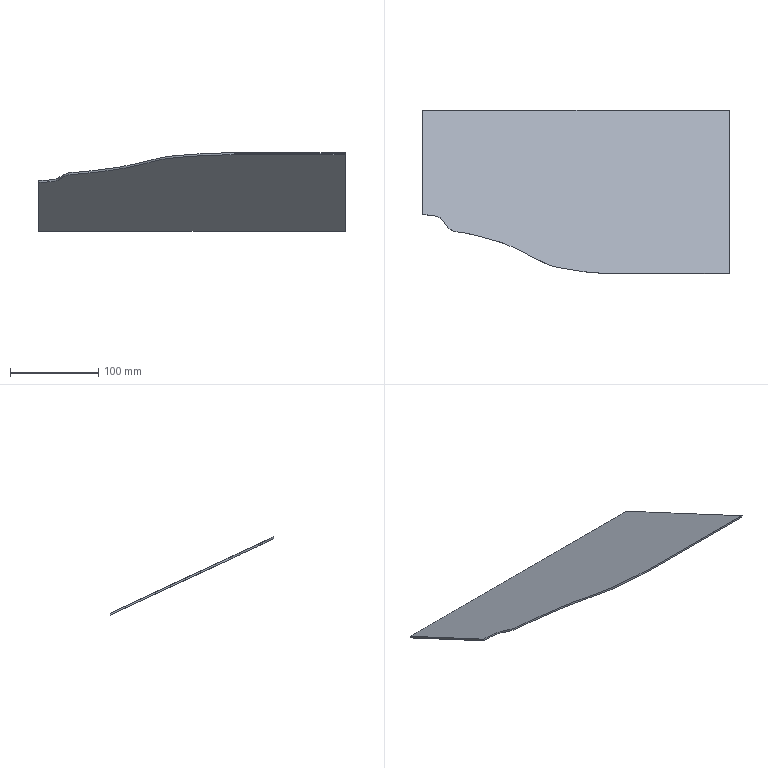Part | NX | features solid 2 | 1 solid | 7 faces | box 347.317 x 185.12 x 88.474 mm | volume 129371 mm3 | plane 6 | spline 1
STEP:
#1=CARTESIAN_POINT('',(-687.317,420.,-186.267));
#2=VERTEX_POINT('',#1);
#3=CARTESIAN_POINT('',(-687.317,420.,-188.474));
#4=VERTEX_POINT('',#3);
#5=CARTESIAN_POINT('',(-687.317,420.,-278.543));
#6=DIRECTION('',(0.,0.,-1.));
#7=VECTOR('',#6,1000.);
#8=LINE('',#5,#7);
#9=EDGE_CURVE('',#2,#4,#8,.T.);
#10=ORIENTED_EDGE('',*,*,#9,.F.);
#11=CARTESIAN_POINT('',(-340.,420.,-186.267));
#12=VERTEX_POINT('',#11);
#13=CARTESIAN_POINT('',(-330.,420.,-186.267));
#14=DIRECTION('',(-1.,0.,0.));
#15=VECTOR('',#14,1000.);
#16=LINE('',#13,#15);
#17=EDGE_CURVE('',#12,#2,#16,.T.);
#18=ORIENTED_EDGE('',*,*,#17,.F.);
#19=CARTESIAN_POINT('',(-340.,420.,-188.474));
#20=VERTEX_POINT('',#19);
#21=CARTESIAN_POINT('',(-340.,420.,10.));
#22=DIRECTION('',(0.,0.,-1.));
#23=VECTOR('',#22,1000.);
#24=LINE('',#21,#23);
#25=EDGE_CURVE('',#12,#20,#24,.T.);
#26=ORIENTED_EDGE('',*,*,#25,.T.);
#27=CARTESIAN_POINT('',(-330.,420.,-188.474));
#28=DIRECTION('',(-1.,0.,0.));
#29=VECTOR('',#28,1000.);
#30=LINE('',#27,#29);
#31=EDGE_CURVE('',#20,#4,#30,.T.);
#32=ORIENTED_EDGE('',*,*,#31,.T.);
#33=EDGE_LOOP('',(#10,#18,#26,#32));
#34=FACE_BOUND('',#33,.T.);
#35=CARTESIAN_POINT('',(0.,420.,10.));
#36=DIRECTION('',(0.,1.,0.));
#37=DIRECTION('',(0.,0.,1.));
#38=AXIS2_PLACEMENT_3D('',#35,#36,#37);
#39=PLANE('',#38);
#40=ADVANCED_FACE('',(#34),#39,.T.);
#41=CARTESIAN_POINT('',(-340.,234.931,-102.175));
#42=VERTEX_POINT('',#41);
#43=CARTESIAN_POINT('',(-340.,234.931,-100.147));
#44=VERTEX_POINT('',#43);
#45=CARTESIAN_POINT('',(-340.,234.931,610.));
#46=DIRECTION('',(0.,0.,-1.));
#47=VECTOR('',#46,1000.);
#48=LINE('',#45,#47);
#49=EDGE_CURVE('',#42,#44,#48,.F.);
#50=ORIENTED_EDGE('',*,*,#49,.F.);
#51=CARTESIAN_POINT('',(-340.,259.69,-113.72));
#52=DIRECTION('',(0.,-0.9063,0.4226));
#53=VECTOR('',#52,1000.);
#54=LINE('',#51,#53);
#55=EDGE_CURVE('',#20,#42,#54,.T.);
#56=ORIENTED_EDGE('',*,*,#55,.F.);
#57=ORIENTED_EDGE('',*,*,#25,.F.);
#58=CARTESIAN_POINT('',(-340.,235.,-100.));
#59=VERTEX_POINT('',#58);
#60=CARTESIAN_POINT('',(-340.,260.535,-111.907));
#61=DIRECTION('',(0.,-0.9063,0.4226));
#62=VECTOR('',#61,1000.);
#63=LINE('',#60,#62);
#64=EDGE_CURVE('',#12,#59,#63,.T.);
#65=ORIENTED_EDGE('',*,*,#64,.T.);
#66=CARTESIAN_POINT('',(-340.,204.395,-165.633));
#67=DIRECTION('',(0.,0.4226,0.9063));
#68=VECTOR('',#67,1000.);
#69=LINE('',#66,#68);
#70=EDGE_CURVE('',#59,#44,#69,.F.);
#71=ORIENTED_EDGE('',*,*,#70,.T.);
#72=EDGE_LOOP('',(#50,#56,#57,#65,#71));
#73=FACE_BOUND('',#72,.T.);
#74=CARTESIAN_POINT('',(-340.,229.93,-177.54));
#75=DIRECTION('',(1.,0.,0.));
#76=DIRECTION('',(0.,1.,0.));
#77=AXIS2_PLACEMENT_3D('',#74,#75,#76);
#78=PLANE('',#77);
#79=ADVANCED_FACE('',(#73),#78,.T.);
#80=CARTESIAN_POINT('',(-480.341,235.,-100.));
#81=VERTEX_POINT('',#80);
#82=CARTESIAN_POINT('',(-340.,234.931,-100.147));
#83=CARTESIAN_POINT('',(-351.695,234.929,-100.153));
#84=CARTESIAN_POINT('',(-369.238,234.931,-100.149));
#85=CARTESIAN_POINT('',(-392.628,234.933,-100.144));
#86=CARTESIAN_POINT('',(-410.171,234.936,-100.138));
#87=CARTESIAN_POINT('',(-427.714,234.923,-100.164));
#88=CARTESIAN_POINT('',(-445.256,234.981,-100.04));
#89=CARTESIAN_POINT('',(-462.799,234.921,-100.169));
#90=CARTESIAN_POINT('',(-474.494,234.863,-100.294));
#91=CARTESIAN_POINT('',(-480.341,235.,-100.));
#92=B_SPLINE_CURVE_WITH_KNOTS('',3,(#82,#83,#84,#85,#86,#87,#88,#89,#90,#91),.UNSPECIFIED.,.F.,.F.,(4,1,1,1,1,1,1,4),(0.,0.03509,0.05263,0.07017,0.08771,0.1053,0.1228,0.1403),.UNSPECIFIED.);
#93=EDGE_CURVE('',#44,#81,#92,.T.);
#94=ORIENTED_EDGE('',*,*,#93,.F.);
#95=ORIENTED_EDGE('',*,*,#70,.F.);
#96=CARTESIAN_POINT('',(-330.,235.,-100.));
#97=DIRECTION('',(-1.,0.,0.));
#98=VECTOR('',#97,1000.);
#99=LINE('',#96,#98);
#100=EDGE_CURVE('',#59,#81,#99,.T.);
#101=ORIENTED_EDGE('',*,*,#100,.T.);
#102=EDGE_LOOP('',(#94,#95,#101));
#103=FACE_BOUND('',#102,.T.);
#104=CARTESIAN_POINT('',(-330.,235.,-100.));
#105=DIRECTION('',(0.,0.9063,-0.4226));
#106=DIRECTION('',(-1.,0.,0.));
#107=AXIS2_PLACEMENT_3D('',#104,#105,#106);
#108=PLANE('',#107);
#109=ADVANCED_FACE('',(#103),#108,.F.);
#110=ORIENTED_EDGE('',*,*,#55,.T.);
#111=CARTESIAN_POINT('',(-687.317,301.902,-133.404));
#112=VERTEX_POINT('',#111);
#113=CARTESIAN_POINT('',(-340.,234.931,-102.175));
#114=CARTESIAN_POINT('',(-355.074,234.928,-102.173));
#115=CARTESIAN_POINT('',(-377.686,234.93,-102.174));
#116=CARTESIAN_POINT('',(-407.834,234.937,-102.178));
#117=CARTESIAN_POINT('',(-430.446,234.919,-102.169));
#118=CARTESIAN_POINT('',(-453.054,235.016,-102.214));
#119=CARTESIAN_POINT('',(-475.676,234.729,-102.08));
#120=CARTESIAN_POINT('',(-494.491,235.465,-102.424));
#121=CARTESIAN_POINT('',(-509.495,237.573,-103.406));
#122=CARTESIAN_POINT('',(-520.718,239.567,-104.336));
#123=CARTESIAN_POINT('',(-532.008,241.304,-105.147));
#124=CARTESIAN_POINT('',(-543.033,243.631,-106.231));
#125=CARTESIAN_POINT('',(-552.986,248.236,-108.379));
#126=CARTESIAN_POINT('',(-562.547,253.682,-110.918));
#127=CARTESIAN_POINT('',(-572.273,258.772,-113.292));
#128=CARTESIAN_POINT('',(-582.129,263.597,-115.542));
#129=CARTESIAN_POINT('',(-592.142,268.098,-117.64));
#130=CARTESIAN_POINT('',(-602.583,271.723,-119.331));
#131=CARTESIAN_POINT('',(-613.442,274.478,-120.616));
#132=CARTESIAN_POINT('',(-622.441,276.919,-121.754));
#133=CARTESIAN_POINT('',(-629.618,278.958,-122.705));
#134=CARTESIAN_POINT('',(-635.058,280.282,-123.322));
#135=CARTESIAN_POINT('',(-640.652,281.056,-123.683));
#136=CARTESIAN_POINT('',(-646.334,281.543,-123.91));
#137=CARTESIAN_POINT('',(-651.889,282.377,-124.299));
#138=CARTESIAN_POINT('',(-657.063,284.955,-125.501));
#139=CARTESIAN_POINT('',(-660.894,289.817,-127.768));
#140=CARTESIAN_POINT('',(-664.331,295.331,-130.34));
#141=CARTESIAN_POINT('',(-668.804,299.109,-132.101));
#142=CARTESIAN_POINT('',(-674.604,300.662,-132.826));
#143=CARTESIAN_POINT('',(-681.069,301.1,-133.03));
#144=CARTESIAN_POINT('',(-685.257,301.597,-133.261));
#145=CARTESIAN_POINT('',(-687.317,301.902,-133.404));
#146=B_SPLINE_CURVE_WITH_KNOTS('',3,(#113,#114,#115,#116,#117,#118,#119,#120,#121,#122,#123,#124,#125,#126,#127,#128,#129,#130,#131,#132,#133,#134,#135,#136,#137,#138,#139,#140,#141,#142,#143,#144,#145),.UNSPECIFIED.,.F.,.F.,(4,1,1,1,1,1,1,1,1,1,1,1,1,1,1,1,1,1,1,1,1,1,1,1,1,1,1,1,1,1,4),(0.,0.0452,0.0678,0.0904,0.113,0.1356,0.1582,0.1695,0.1808,0.1921,0.2034,0.2147,0.226,0.2373,0.2486,0.2599,0.2712,0.2825,0.2938,0.2994,0.3051,0.3107,0.3164,0.322,0.3277,0.3333,0.339,0.3446,0.3503,0.3559,0.3616),.UNSPECIFIED.);
#147=EDGE_CURVE('',#42,#112,#146,.T.);
#148=ORIENTED_EDGE('',*,*,#147,.T.);
#149=CARTESIAN_POINT('',(-687.317,596.678,-270.86));
#150=DIRECTION('',(0.,-0.9063,0.4226));
#151=VECTOR('',#150,1000.);
#152=LINE('',#149,#151);
#153=EDGE_CURVE('',#4,#112,#152,.T.);
#154=ORIENTED_EDGE('',*,*,#153,.F.);
#155=ORIENTED_EDGE('',*,*,#31,.F.);
#156=EDGE_LOOP('',(#110,#148,#154,#155));
#157=FACE_BOUND('',#156,.T.);
#158=CARTESIAN_POINT('',(-330.,596.678,-270.86));
#159=DIRECTION('',(0.,0.4226,0.9063));
#160=DIRECTION('',(1.,0.,0.));
#161=AXIS2_PLACEMENT_3D('',#158,#159,#160);
#162=PLANE('',#161);
#163=ADVANCED_FACE('',(#157),#162,.F.);
#164=CARTESIAN_POINT('',(-687.317,301.902,-131.197));
#165=VERTEX_POINT('',#164);
#166=CARTESIAN_POINT('',(-687.317,301.902,-133.808));
#167=DIRECTION('',(0.,0.,-1.));
#168=VECTOR('',#167,1000.);
#169=LINE('',#166,#168);
#170=EDGE_CURVE('',#165,#112,#169,.T.);
#171=ORIENTED_EDGE('',*,*,#170,.F.);
#172=CARTESIAN_POINT('',(-687.317,597.523,-269.047));
#173=DIRECTION('',(0.,-0.9063,0.4226));
#174=VECTOR('',#173,1000.);
#175=LINE('',#172,#174);
#176=EDGE_CURVE('',#2,#165,#175,.T.);
#177=ORIENTED_EDGE('',*,*,#176,.F.);
#178=ORIENTED_EDGE('',*,*,#9,.T.);
#179=ORIENTED_EDGE('',*,*,#153,.T.);
#180=EDGE_LOOP('',(#171,#177,#178,#179));
#181=FACE_BOUND('',#180,.T.);
#182=CARTESIAN_POINT('',(-687.317,415.853,-278.543));
#183=DIRECTION('',(-1.,0.,0.));
#184=DIRECTION('',(0.,0.,1.));
#185=AXIS2_PLACEMENT_3D('',#182,#183,#184);
#186=PLANE('',#185);
#187=ADVANCED_FACE('',(#181),#186,.T.);
#188=CARTESIAN_POINT('',(-480.341,235.,-100.));
#189=CARTESIAN_POINT('',(-485.184,235.114,-100.053));
#190=CARTESIAN_POINT('',(-494.831,235.59,-100.275));
#191=CARTESIAN_POINT('',(-509.128,237.47,-101.152));
#192=CARTESIAN_POINT('',(-520.955,239.594,-102.142));
#193=CARTESIAN_POINT('',(-530.45,241.116,-102.852));
#194=CARTESIAN_POINT('',(-537.531,242.404,-103.453));
#195=CARTESIAN_POINT('',(-544.264,244.33,-104.351));
#196=CARTESIAN_POINT('',(-550.56,247.084,-105.635));
#197=CARTESIAN_POINT('',(-556.599,250.322,-107.145));
#198=CARTESIAN_POINT('',(-564.584,254.766,-109.217));
#199=CARTESIAN_POINT('',(-574.719,260.029,-111.671));
#200=CARTESIAN_POINT('',(-587.087,265.966,-114.44));
#201=CARTESIAN_POINT('',(-599.843,271.007,-116.79));
#202=CARTESIAN_POINT('',(-611.053,273.879,-118.13));
#203=CARTESIAN_POINT('',(-620.004,276.226,-119.224));
#204=CARTESIAN_POINT('',(-626.681,278.134,-120.114));
#205=CARTESIAN_POINT('',(-633.375,279.968,-120.969));
#206=CARTESIAN_POINT('',(-640.261,281.063,-121.48));
#207=CARTESIAN_POINT('',(-647.289,281.562,-121.712));
#208=CARTESIAN_POINT('',(-652.977,282.75,-122.266));
#209=CARTESIAN_POINT('',(-656.843,285.163,-123.391));
#210=CARTESIAN_POINT('',(-659.875,288.303,-124.856));
#211=CARTESIAN_POINT('',(-662.704,292.92,-127.009));
#212=CARTESIAN_POINT('',(-666.161,297.202,-129.005));
#213=CARTESIAN_POINT('',(-670.181,299.408,-130.034));
#214=CARTESIAN_POINT('',(-674.613,300.635,-130.606));
#215=CARTESIAN_POINT('',(-680.434,301.053,-130.801));
#216=CARTESIAN_POINT('',(-685.03,301.563,-131.039));
#217=CARTESIAN_POINT('',(-687.317,301.902,-131.197));
#218=B_SPLINE_CURVE_WITH_KNOTS('',3,(#188,#189,#190,#191,#192,#193,#194,#195,#196,#197,#198,#199,#200,#201,#202,#203,#204,#205,#206,#207,#208,#209,#210,#211,#212,#213,#214,#215,#216,#217),.UNSPECIFIED.,.F.,.F.,(4,1,1,1,1,1,1,1,1,1,1,1,1,1,1,1,1,1,1,1,1,1,1,1,1,1,1,4),(0.,0.01445,0.02889,0.04334,0.05056,0.05778,0.065,0.07223,0.07945,0.08667,0.1011,0.1156,0.13,0.1445,0.1517,0.1589,0.1661,0.1733,0.1806,0.1878,0.1914,0.195,0.2022,0.2095,0.2131,0.2167,0.2239,0.2311),.UNSPECIFIED.);
#219=EDGE_CURVE('',#81,#165,#218,.T.);
#220=ORIENTED_EDGE('',*,*,#219,.F.);
#221=ORIENTED_EDGE('',*,*,#100,.F.);
#222=ORIENTED_EDGE('',*,*,#64,.F.);
#223=ORIENTED_EDGE('',*,*,#17,.T.);
#224=ORIENTED_EDGE('',*,*,#176,.T.);
#225=EDGE_LOOP('',(#220,#221,#222,#223,#224));
#226=FACE_BOUND('',#225,.T.);
#227=CARTESIAN_POINT('',(-330.,597.523,-269.047));
#228=DIRECTION('',(0.,0.4226,0.9063));
#229=DIRECTION('',(1.,0.,0.));
#230=AXIS2_PLACEMENT_3D('',#227,#228,#229);
#231=PLANE('',#230);
#232=ADVANCED_FACE('',(#226),#231,.T.);
#233=ORIENTED_EDGE('',*,*,#49,.T.);
#234=ORIENTED_EDGE('',*,*,#93,.T.);
#235=ORIENTED_EDGE('',*,*,#219,.T.);
#236=ORIENTED_EDGE('',*,*,#170,.T.);
#237=ORIENTED_EDGE('',*,*,#147,.F.);
#238=EDGE_LOOP('',(#233,#234,#235,#236,#237));
#239=FACE_BOUND('',#238,.T.);
#240=CARTESIAN_POINT('',(-687.317,301.902,-99.784));
#241=CARTESIAN_POINT('',(-687.317,301.902,-133.604));
#242=CARTESIAN_POINT('',(-685.448,301.625,-99.784));
#243=CARTESIAN_POINT('',(-685.448,301.625,-133.604));
#244=CARTESIAN_POINT('',(-681.696,301.156,-99.784));
#245=CARTESIAN_POINT('',(-681.696,301.156,-133.604));
#246=CARTESIAN_POINT('',(-676.029,300.788,-99.784));
#247=CARTESIAN_POINT('',(-676.029,300.788,-133.604));
#248=CARTESIAN_POINT('',(-671.358,299.89,-99.784));
#249=CARTESIAN_POINT('',(-671.358,299.89,-133.604));
#250=CARTESIAN_POINT('',(-667.944,298.244,-99.784));
#251=CARTESIAN_POINT('',(-667.944,298.244,-133.604));
#252=CARTESIAN_POINT('',(-664.976,295.856,-99.784));
#253=CARTESIAN_POINT('',(-664.976,295.856,-133.604));
#254=CARTESIAN_POINT('',(-662.201,292.036,-99.784));
#255=CARTESIAN_POINT('',(-662.201,292.036,-133.604));
#256=CARTESIAN_POINT('',(-659.62,288.033,-99.784));
#257=CARTESIAN_POINT('',(-659.62,288.033,-133.604));
#258=CARTESIAN_POINT('',(-656.978,285.322,-99.784));
#259=CARTESIAN_POINT('',(-656.978,285.322,-133.604));
#260=CARTESIAN_POINT('',(-653.811,283.203,-99.784));
#261=CARTESIAN_POINT('',(-653.811,283.203,-133.604));
#262=CARTESIAN_POINT('',(-649.284,281.841,-99.784));
#263=CARTESIAN_POINT('',(-649.284,281.841,-133.604));
#264=CARTESIAN_POINT('',(-643.58,281.33,-99.784));
#265=CARTESIAN_POINT('',(-643.58,281.33,-133.604));
#266=CARTESIAN_POINT('',(-637.943,280.742,-99.784));
#267=CARTESIAN_POINT('',(-637.943,280.742,-133.604));
#268=CARTESIAN_POINT('',(-632.389,279.692,-99.784));
#269=CARTESIAN_POINT('',(-632.389,279.692,-133.604));
#270=CARTESIAN_POINT('',(-625.084,277.691,-99.784));
#271=CARTESIAN_POINT('',(-625.084,277.691,-133.604));
#272=CARTESIAN_POINT('',(-616.002,275.107,-99.784));
#273=CARTESIAN_POINT('',(-616.002,275.107,-133.604));
#274=CARTESIAN_POINT('',(-604.99,272.392,-99.784));
#275=CARTESIAN_POINT('',(-604.99,272.392,-133.604));
#276=CARTESIAN_POINT('',(-594.187,268.925,-99.784));
#277=CARTESIAN_POINT('',(-594.187,268.925,-133.604));
#278=CARTESIAN_POINT('',(-583.79,264.382,-99.784));
#279=CARTESIAN_POINT('',(-583.79,264.382,-133.604));
#280=CARTESIAN_POINT('',(-573.588,259.44,-99.784));
#281=CARTESIAN_POINT('',(-573.588,259.44,-133.604));
#282=CARTESIAN_POINT('',(-563.521,254.219,-99.784));
#283=CARTESIAN_POINT('',(-563.521,254.219,-133.604));
#284=CARTESIAN_POINT('',(-553.676,248.612,-99.784));
#285=CARTESIAN_POINT('',(-553.676,248.612,-133.604));
#286=CARTESIAN_POINT('',(-543.396,243.726,-99.784));
#287=CARTESIAN_POINT('',(-543.396,243.726,-133.604));
#288=CARTESIAN_POINT('',(-532.263,241.342,-99.784));
#289=CARTESIAN_POINT('',(-532.263,241.342,-133.604));
#290=CARTESIAN_POINT('',(-521.066,239.627,-99.784));
#291=CARTESIAN_POINT('',(-521.066,239.627,-133.604));
#292=CARTESIAN_POINT('',(-509.899,237.642,-99.784));
#293=CARTESIAN_POINT('',(-509.899,237.642,-133.604));
#294=CARTESIAN_POINT('',(-494.935,235.503,-99.784));
#295=CARTESIAN_POINT('',(-494.935,235.503,-133.604));
#296=CARTESIAN_POINT('',(-476.032,234.723,-99.784));
#297=CARTESIAN_POINT('',(-476.032,234.723,-133.604));
#298=CARTESIAN_POINT('',(-453.361,235.016,-99.784));
#299=CARTESIAN_POINT('',(-453.361,235.016,-133.604));
#300=CARTESIAN_POINT('',(-430.689,234.919,-99.784));
#301=CARTESIAN_POINT('',(-430.689,234.919,-133.604));
#302=CARTESIAN_POINT('',(-408.017,234.937,-99.784));
#303=CARTESIAN_POINT('',(-408.017,234.937,-133.604));
#304=CARTESIAN_POINT('',(-377.787,234.93,-99.784));
#305=CARTESIAN_POINT('',(-377.787,234.93,-133.604));
#306=CARTESIAN_POINT('',(-355.115,234.928,-99.784));
#307=CARTESIAN_POINT('',(-355.115,234.928,-133.604));
#308=CARTESIAN_POINT('',(-340.,234.931,-99.784));
#309=CARTESIAN_POINT('',(-340.,234.931,-133.604));
#310=B_SPLINE_SURFACE_WITH_KNOTS('',3,1,((#240,#241),(#242,#243),(#244,#245),(#246,#247),(#248,#249),(#250,#251),(#252,#253),(#254,#255),(#256,#257),(#258,#259),(#260,#261),(#262,#263),(#264,#265),(#266,#267),(#268,#269),(#270,#271),(#272,#273),(#274,#275),(#276,#277),(#278,#279),(#280,#281),(#282,#283),(#284,#285),(#286,#287),(#288,#289),(#290,#291),(#292,#293),(#294,#295),(#296,#297),(#298,#299),(#300,#301),(#302,#303),(#304,#305),(#306,#307),(#308,#309)),.SURF_OF_LINEAR_EXTRUSION.,.F.,.F.,.F.,(4,1,1,1,1,1,1,1,1,1,1,1,1,1,1,1,1,1,1,1,1,1,1,1,1,1,1,1,1,1,1,1,4),(2,2),(0.5435,0.5448,0.546,0.5473,0.5479,0.5485,0.5498,0.551,0.5516,0.5523,0.5535,0.5548,0.556,0.5572,0.5585,0.561,0.5635,0.566,0.5685,0.571,0.5735,0.5759,0.5784,0.5809,0.5834,0.5859,0.5884,0.5934,0.5984,0.6034,0.6084,0.6133,0.6233),(0.,1.),.UNSPECIFIED.);
#311=ADVANCED_FACE('',(#239),#310,.F.);
#312=CLOSED_SHELL('',(#40,#79,#109,#163,#187,#232,#311));
#313=MANIFOLD_SOLID_BREP('',#312);
#314=(LENGTH_UNIT()NAMED_UNIT(*)SI_UNIT(.MILLI.,.METRE.));
#315=UNCERTAINTY_MEASURE_WITH_UNIT(LENGTH_MEASURE(0.0508),#314,'','');
#316=(NAMED_UNIT(*)PLANE_ANGLE_UNIT()SI_UNIT($,.RADIAN.));
#317=(NAMED_UNIT(*)SI_UNIT($,.STERADIAN.)SOLID_ANGLE_UNIT());
#318=(GEOMETRIC_REPRESENTATION_CONTEXT(3)GLOBAL_UNCERTAINTY_ASSIGNED_CONTEXT((#315))GLOBAL_UNIT_ASSIGNED_CONTEXT((#314,#316,#317))REPRESENTATION_CONTEXT('',''));
#319=ADVANCED_BREP_SHAPE_REPRESENTATION('',(#313),#318);